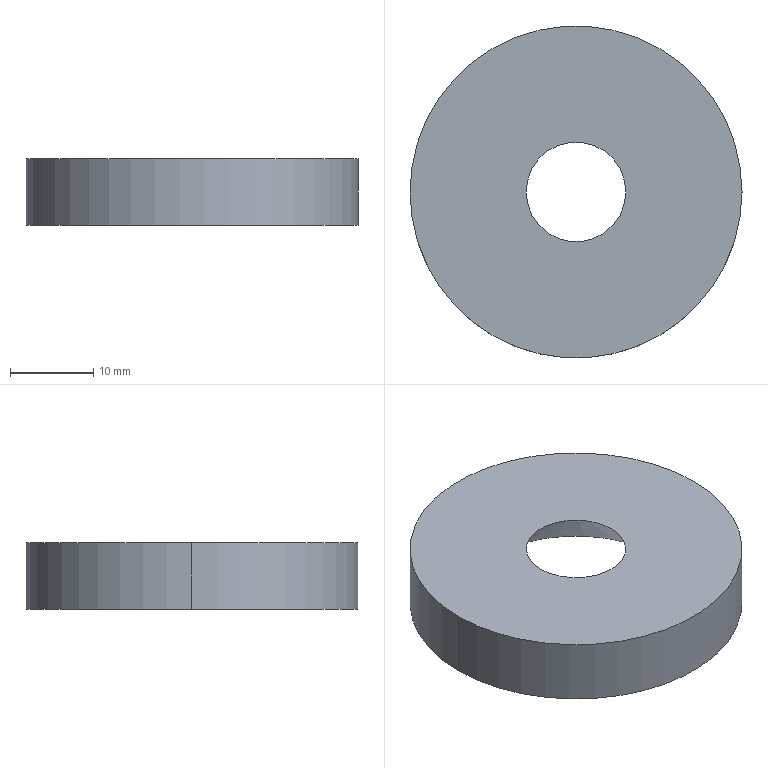Part | STEP file | 1 solid | 6 faces | box 40 x 40 x 8 mm | volume 7406 mm3 | cone 2 | plane 2 | cylinder 2 | commonest cylinder face diameters 40 x2
STEP:
#1=CARTESIAN_POINT('',(0.,0.,0.));
#2=DIRECTION('',(0.,0.,1.));
#3=DIRECTION('',(1.,0.,0.));
#4=AXIS2_PLACEMENT_3D('',#1,#2,#3);
#5=CARTESIAN_POINT('',(-14.,0.,0.));
#6=VERTEX_POINT('',#5);
#7=CARTESIAN_POINT('',(14.,0.,0.));
#8=VERTEX_POINT('',#7);
#9=CARTESIAN_POINT('',(0.,0.,0.));
#10=DIRECTION('',(0.,0.,1.));
#11=DIRECTION('',(1.,0.,0.));
#12=AXIS2_PLACEMENT_3D('',#9,#10,#11);
#13=CIRCLE('',#12,14.);
#14=CARTESIAN_POINT('',(0.,0.,8.));
#15=DIRECTION('',(0.,0.,-1.));
#16=DIRECTION('',(1.,0.,0.));
#17=AXIS2_PLACEMENT_3D('',#14,#15,#16);
#18=CONICAL_SURFACE('',#17,6.,0.7854);
#19=CARTESIAN_POINT('',(6.283,8.));
#20=DIRECTION('',(-1.,0.));
#21=VECTOR('',#20,1.);
#22=LINE('',#19,#21);
#23=(GEOMETRIC_REPRESENTATION_CONTEXT(2)PARAMETRIC_REPRESENTATION_CONTEXT()REPRESENTATION_CONTEXT('',''));
#24=DEFINITIONAL_REPRESENTATION('',(#22),#23);
#25=PCURVE('',#18,#24);
#26=CARTESIAN_POINT('',(0.,0.,0.));
#27=DIRECTION('',(0.,0.,1.));
#28=DIRECTION('',(1.,0.,0.));
#29=AXIS2_PLACEMENT_3D('',#26,#27,#28);
#30=PLANE('',#29);
#31=CARTESIAN_POINT('',(0.,0.));
#32=DIRECTION('',(1.,0.));
#33=AXIS2_PLACEMENT_2D('',#31,#32);
#34=CIRCLE('',#33,14.);
#35=(GEOMETRIC_REPRESENTATION_CONTEXT(2)PARAMETRIC_REPRESENTATION_CONTEXT()REPRESENTATION_CONTEXT('',''));
#36=DEFINITIONAL_REPRESENTATION('',(#34),#35);
#37=PCURVE('',#30,#36);
#38=SURFACE_CURVE('',#13,(#25,#37),.PCURVE_S1.);
#39=EDGE_CURVE('',#6,#8,#38,.T.);
#40=ORIENTED_EDGE('',*,*,#39,.T.);
#41=CARTESIAN_POINT('',(6.,0.,8.));
#42=VERTEX_POINT('',#41);
#43=CARTESIAN_POINT('',(6.,0.,8.));
#44=DIRECTION('',(0.7071,0.,-0.7071));
#45=VECTOR('',#44,1.);
#46=LINE('',#43,#45);
#47=CARTESIAN_POINT('',(0.,0.));
#48=DIRECTION('',(0.,1.));
#49=VECTOR('',#48,1.);
#50=LINE('',#47,#49);
#51=(GEOMETRIC_REPRESENTATION_CONTEXT(2)PARAMETRIC_REPRESENTATION_CONTEXT()REPRESENTATION_CONTEXT('',''));
#52=DEFINITIONAL_REPRESENTATION('',(#50),#51);
#53=PCURVE('',#18,#52);
#54=CARTESIAN_POINT('',(0.,0.,8.));
#55=DIRECTION('',(0.,0.,-1.));
#56=DIRECTION('',(1.,0.,0.));
#57=AXIS2_PLACEMENT_3D('',#54,#55,#56);
#58=CONICAL_SURFACE('',#57,6.,0.7854);
#59=CARTESIAN_POINT('',(6.283,0.));
#60=DIRECTION('',(0.,1.));
#61=VECTOR('',#60,1.);
#62=LINE('',#59,#61);
#63=(GEOMETRIC_REPRESENTATION_CONTEXT(2)PARAMETRIC_REPRESENTATION_CONTEXT()REPRESENTATION_CONTEXT('',''));
#64=DEFINITIONAL_REPRESENTATION('',(#62),#63);
#65=PCURVE('',#58,#64);
#66=SURFACE_CURVE('',#46,(#53,#65),.PCURVE_S1.);
#67=EDGE_CURVE('',#42,#8,#66,.T.);
#68=ORIENTED_EDGE('',*,*,#67,.F.);
#69=CARTESIAN_POINT('',(-6.,0.,8.));
#70=VERTEX_POINT('',#69);
#71=CARTESIAN_POINT('',(0.,0.,8.));
#72=DIRECTION('',(0.,0.,1.));
#73=DIRECTION('',(1.,0.,0.));
#74=AXIS2_PLACEMENT_3D('',#71,#72,#73);
#75=CIRCLE('',#74,6.);
#76=CARTESIAN_POINT('',(6.283,0.));
#77=DIRECTION('',(-1.,0.));
#78=VECTOR('',#77,1.);
#79=LINE('',#76,#78);
#80=(GEOMETRIC_REPRESENTATION_CONTEXT(2)PARAMETRIC_REPRESENTATION_CONTEXT()REPRESENTATION_CONTEXT('',''));
#81=DEFINITIONAL_REPRESENTATION('',(#79),#80);
#82=PCURVE('',#18,#81);
#83=CARTESIAN_POINT('',(0.,0.,8.));
#84=DIRECTION('',(0.,0.,1.));
#85=DIRECTION('',(1.,0.,0.));
#86=AXIS2_PLACEMENT_3D('',#83,#84,#85);
#87=PLANE('',#86);
#88=CARTESIAN_POINT('',(0.,0.));
#89=DIRECTION('',(1.,0.));
#90=AXIS2_PLACEMENT_2D('',#88,#89);
#91=CIRCLE('',#90,6.);
#92=(GEOMETRIC_REPRESENTATION_CONTEXT(2)PARAMETRIC_REPRESENTATION_CONTEXT()REPRESENTATION_CONTEXT('',''));
#93=DEFINITIONAL_REPRESENTATION('',(#91),#92);
#94=PCURVE('',#87,#93);
#95=SURFACE_CURVE('',#75,(#82,#94),.PCURVE_S1.);
#96=EDGE_CURVE('',#70,#42,#95,.T.);
#97=ORIENTED_EDGE('',*,*,#96,.F.);
#98=CARTESIAN_POINT('',(-6.,0.,8.));
#99=DIRECTION('',(-0.7071,0.,-0.7071));
#100=VECTOR('',#99,1.);
#101=LINE('',#98,#100);
#102=CARTESIAN_POINT('',(3.142,0.));
#103=DIRECTION('',(0.,1.));
#104=VECTOR('',#103,1.);
#105=LINE('',#102,#104);
#106=(GEOMETRIC_REPRESENTATION_CONTEXT(2)PARAMETRIC_REPRESENTATION_CONTEXT()REPRESENTATION_CONTEXT('',''));
#107=DEFINITIONAL_REPRESENTATION('',(#105),#106);
#108=PCURVE('',#18,#107);
#109=CARTESIAN_POINT('',(3.142,0.));
#110=DIRECTION('',(0.,1.));
#111=VECTOR('',#110,1.);
#112=LINE('',#109,#111);
#113=(GEOMETRIC_REPRESENTATION_CONTEXT(2)PARAMETRIC_REPRESENTATION_CONTEXT()REPRESENTATION_CONTEXT('',''));
#114=DEFINITIONAL_REPRESENTATION('',(#112),#113);
#115=PCURVE('',#58,#114);
#116=SURFACE_CURVE('',#101,(#108,#115),.PCURVE_S1.);
#117=EDGE_CURVE('',#70,#6,#116,.T.);
#118=ORIENTED_EDGE('',*,*,#117,.T.);
#119=EDGE_LOOP('',(#40,#68,#97,#118));
#120=FACE_BOUND('',#119,.F.);
#121=ADVANCED_FACE('',(#120),#18,.F.);
#122=CARTESIAN_POINT('',(0.,0.,0.));
#123=DIRECTION('',(0.,0.,1.));
#124=DIRECTION('',(1.,0.,0.));
#125=AXIS2_PLACEMENT_3D('',#122,#123,#124);
#126=CIRCLE('',#125,14.);
#127=CARTESIAN_POINT('',(0.,0.));
#128=DIRECTION('',(1.,0.));
#129=AXIS2_PLACEMENT_2D('',#127,#128);
#130=CIRCLE('',#129,14.);
#131=(GEOMETRIC_REPRESENTATION_CONTEXT(2)PARAMETRIC_REPRESENTATION_CONTEXT()REPRESENTATION_CONTEXT('',''));
#132=DEFINITIONAL_REPRESENTATION('',(#130),#131);
#133=PCURVE('',#30,#132);
#134=CARTESIAN_POINT('',(6.283,8.));
#135=DIRECTION('',(-1.,0.));
#136=VECTOR('',#135,1.);
#137=LINE('',#134,#136);
#138=(GEOMETRIC_REPRESENTATION_CONTEXT(2)PARAMETRIC_REPRESENTATION_CONTEXT()REPRESENTATION_CONTEXT('',''));
#139=DEFINITIONAL_REPRESENTATION('',(#137),#138);
#140=PCURVE('',#58,#139);
#141=SURFACE_CURVE('',#126,(#133,#140),.PCURVE_S1.);
#142=EDGE_CURVE('',#8,#6,#141,.T.);
#143=ORIENTED_EDGE('',*,*,#142,.T.);
#144=ORIENTED_EDGE('',*,*,#39,.T.);
#145=EDGE_LOOP('',(#143,#144));
#146=FACE_BOUND('',#145,.T.);
#147=CARTESIAN_POINT('',(-20.,0.,0.));
#148=VERTEX_POINT('',#147);
#149=CARTESIAN_POINT('',(20.,0.,0.));
#150=VERTEX_POINT('',#149);
#151=CARTESIAN_POINT('',(0.,0.,0.));
#152=DIRECTION('',(0.,0.,1.));
#153=DIRECTION('',(1.,0.,0.));
#154=AXIS2_PLACEMENT_3D('',#151,#152,#153);
#155=CIRCLE('',#154,20.);
#156=CARTESIAN_POINT('',(0.,0.));
#157=DIRECTION('',(1.,0.));
#158=AXIS2_PLACEMENT_2D('',#156,#157);
#159=CIRCLE('',#158,20.);
#160=(GEOMETRIC_REPRESENTATION_CONTEXT(2)PARAMETRIC_REPRESENTATION_CONTEXT()REPRESENTATION_CONTEXT('',''));
#161=DEFINITIONAL_REPRESENTATION('',(#159),#160);
#162=PCURVE('',#30,#161);
#163=CARTESIAN_POINT('',(0.,0.,8.));
#164=DIRECTION('',(0.,0.,-1.));
#165=DIRECTION('',(-1.,0.,0.));
#166=AXIS2_PLACEMENT_3D('',#163,#164,#165);
#167=CYLINDRICAL_SURFACE('',#166,20.);
#168=CARTESIAN_POINT('',(9.425,8.));
#169=DIRECTION('',(-1.,0.));
#170=VECTOR('',#169,1.);
#171=LINE('',#168,#170);
#172=(GEOMETRIC_REPRESENTATION_CONTEXT(2)PARAMETRIC_REPRESENTATION_CONTEXT()REPRESENTATION_CONTEXT('',''));
#173=DEFINITIONAL_REPRESENTATION('',(#171),#172);
#174=PCURVE('',#167,#173);
#175=SURFACE_CURVE('',#155,(#162,#174),.PCURVE_S1.);
#176=EDGE_CURVE('',#148,#150,#175,.T.);
#177=ORIENTED_EDGE('',*,*,#176,.F.);
#178=CARTESIAN_POINT('',(0.,0.,0.));
#179=DIRECTION('',(0.,0.,1.));
#180=DIRECTION('',(1.,0.,0.));
#181=AXIS2_PLACEMENT_3D('',#178,#179,#180);
#182=CIRCLE('',#181,20.);
#183=CARTESIAN_POINT('',(0.,0.));
#184=DIRECTION('',(1.,0.));
#185=AXIS2_PLACEMENT_2D('',#183,#184);
#186=CIRCLE('',#185,20.);
#187=(GEOMETRIC_REPRESENTATION_CONTEXT(2)PARAMETRIC_REPRESENTATION_CONTEXT()REPRESENTATION_CONTEXT('',''));
#188=DEFINITIONAL_REPRESENTATION('',(#186),#187);
#189=PCURVE('',#30,#188);
#190=CARTESIAN_POINT('',(0.,0.,8.));
#191=DIRECTION('',(0.,0.,-1.));
#192=DIRECTION('',(-1.,0.,0.));
#193=AXIS2_PLACEMENT_3D('',#190,#191,#192);
#194=CYLINDRICAL_SURFACE('',#193,20.);
#195=CARTESIAN_POINT('',(3.142,8.));
#196=DIRECTION('',(-1.,0.));
#197=VECTOR('',#196,1.);
#198=LINE('',#195,#197);
#199=(GEOMETRIC_REPRESENTATION_CONTEXT(2)PARAMETRIC_REPRESENTATION_CONTEXT()REPRESENTATION_CONTEXT('',''));
#200=DEFINITIONAL_REPRESENTATION('',(#198),#199);
#201=PCURVE('',#194,#200);
#202=SURFACE_CURVE('',#182,(#189,#201),.PCURVE_S1.);
#203=EDGE_CURVE('',#150,#148,#202,.T.);
#204=ORIENTED_EDGE('',*,*,#203,.F.);
#205=EDGE_LOOP('',(#177,#204));
#206=FACE_BOUND('',#205,.T.);
#207=ADVANCED_FACE('',(#146,#206),#30,.F.);
#208=CARTESIAN_POINT('',(0.,0.,8.));
#209=DIRECTION('',(0.,0.,1.));
#210=DIRECTION('',(1.,0.,0.));
#211=AXIS2_PLACEMENT_3D('',#208,#209,#210);
#212=CIRCLE('',#211,6.);
#213=CARTESIAN_POINT('',(0.,0.));
#214=DIRECTION('',(1.,0.));
#215=AXIS2_PLACEMENT_2D('',#213,#214);
#216=CIRCLE('',#215,6.);
#217=(GEOMETRIC_REPRESENTATION_CONTEXT(2)PARAMETRIC_REPRESENTATION_CONTEXT()REPRESENTATION_CONTEXT('',''));
#218=DEFINITIONAL_REPRESENTATION('',(#216),#217);
#219=PCURVE('',#87,#218);
#220=CARTESIAN_POINT('',(6.283,0.));
#221=DIRECTION('',(-1.,0.));
#222=VECTOR('',#221,1.);
#223=LINE('',#220,#222);
#224=(GEOMETRIC_REPRESENTATION_CONTEXT(2)PARAMETRIC_REPRESENTATION_CONTEXT()REPRESENTATION_CONTEXT('',''));
#225=DEFINITIONAL_REPRESENTATION('',(#223),#224);
#226=PCURVE('',#58,#225);
#227=SURFACE_CURVE('',#212,(#219,#226),.PCURVE_S1.);
#228=EDGE_CURVE('',#42,#70,#227,.T.);
#229=ORIENTED_EDGE('',*,*,#228,.F.);
#230=ORIENTED_EDGE('',*,*,#96,.F.);
#231=EDGE_LOOP('',(#229,#230));
#232=FACE_BOUND('',#231,.T.);
#233=CARTESIAN_POINT('',(-20.,0.,8.));
#234=VERTEX_POINT('',#233);
#235=CARTESIAN_POINT('',(20.,0.,8.));
#236=VERTEX_POINT('',#235);
#237=CARTESIAN_POINT('',(0.,0.,8.));
#238=DIRECTION('',(0.,0.,1.));
#239=DIRECTION('',(1.,0.,0.));
#240=AXIS2_PLACEMENT_3D('',#237,#238,#239);
#241=CIRCLE('',#240,20.);
#242=CARTESIAN_POINT('',(0.,0.));
#243=DIRECTION('',(1.,0.));
#244=AXIS2_PLACEMENT_2D('',#242,#243);
#245=CIRCLE('',#244,20.);
#246=(GEOMETRIC_REPRESENTATION_CONTEXT(2)PARAMETRIC_REPRESENTATION_CONTEXT()REPRESENTATION_CONTEXT('',''));
#247=DEFINITIONAL_REPRESENTATION('',(#245),#246);
#248=PCURVE('',#87,#247);
#249=CARTESIAN_POINT('',(9.425,0.));
#250=DIRECTION('',(-1.,0.));
#251=VECTOR('',#250,1.);
#252=LINE('',#249,#251);
#253=(GEOMETRIC_REPRESENTATION_CONTEXT(2)PARAMETRIC_REPRESENTATION_CONTEXT()REPRESENTATION_CONTEXT('',''));
#254=DEFINITIONAL_REPRESENTATION('',(#252),#253);
#255=PCURVE('',#167,#254);
#256=SURFACE_CURVE('',#241,(#248,#255),.PCURVE_S1.);
#257=EDGE_CURVE('',#234,#236,#256,.T.);
#258=ORIENTED_EDGE('',*,*,#257,.T.);
#259=CARTESIAN_POINT('',(0.,0.,8.));
#260=DIRECTION('',(0.,0.,1.));
#261=DIRECTION('',(1.,0.,0.));
#262=AXIS2_PLACEMENT_3D('',#259,#260,#261);
#263=CIRCLE('',#262,20.);
#264=CARTESIAN_POINT('',(0.,0.));
#265=DIRECTION('',(1.,0.));
#266=AXIS2_PLACEMENT_2D('',#264,#265);
#267=CIRCLE('',#266,20.);
#268=(GEOMETRIC_REPRESENTATION_CONTEXT(2)PARAMETRIC_REPRESENTATION_CONTEXT()REPRESENTATION_CONTEXT('',''));
#269=DEFINITIONAL_REPRESENTATION('',(#267),#268);
#270=PCURVE('',#87,#269);
#271=CARTESIAN_POINT('',(3.142,0.));
#272=DIRECTION('',(-1.,0.));
#273=VECTOR('',#272,1.);
#274=LINE('',#271,#273);
#275=(GEOMETRIC_REPRESENTATION_CONTEXT(2)PARAMETRIC_REPRESENTATION_CONTEXT()REPRESENTATION_CONTEXT('',''));
#276=DEFINITIONAL_REPRESENTATION('',(#274),#275);
#277=PCURVE('',#194,#276);
#278=SURFACE_CURVE('',#263,(#270,#277),.PCURVE_S1.);
#279=EDGE_CURVE('',#236,#234,#278,.T.);
#280=ORIENTED_EDGE('',*,*,#279,.T.);
#281=EDGE_LOOP('',(#258,#280));
#282=FACE_BOUND('',#281,.T.);
#283=ADVANCED_FACE('',(#232,#282),#87,.T.);
#284=CARTESIAN_POINT('',(20.,0.,8.));
#285=DIRECTION('',(0.,0.,-1.));
#286=VECTOR('',#285,1.);
#287=LINE('',#284,#286);
#288=CARTESIAN_POINT('',(3.142,0.));
#289=DIRECTION('',(0.,1.));
#290=VECTOR('',#289,1.);
#291=LINE('',#288,#290);
#292=(GEOMETRIC_REPRESENTATION_CONTEXT(2)PARAMETRIC_REPRESENTATION_CONTEXT()REPRESENTATION_CONTEXT('',''));
#293=DEFINITIONAL_REPRESENTATION('',(#291),#292);
#294=PCURVE('',#167,#293);
#295=CARTESIAN_POINT('',(3.142,0.));
#296=DIRECTION('',(0.,1.));
#297=VECTOR('',#296,1.);
#298=LINE('',#295,#297);
#299=(GEOMETRIC_REPRESENTATION_CONTEXT(2)PARAMETRIC_REPRESENTATION_CONTEXT()REPRESENTATION_CONTEXT('',''));
#300=DEFINITIONAL_REPRESENTATION('',(#298),#299);
#301=PCURVE('',#194,#300);
#302=SURFACE_CURVE('',#287,(#294,#301),.PCURVE_S1.);
#303=EDGE_CURVE('',#236,#150,#302,.T.);
#304=ORIENTED_EDGE('',*,*,#303,.F.);
#305=ORIENTED_EDGE('',*,*,#257,.F.);
#306=CARTESIAN_POINT('',(-20.,0.,8.));
#307=DIRECTION('',(0.,0.,-1.));
#308=VECTOR('',#307,1.);
#309=LINE('',#306,#308);
#310=CARTESIAN_POINT('',(6.283,0.));
#311=DIRECTION('',(0.,1.));
#312=VECTOR('',#311,1.);
#313=LINE('',#310,#312);
#314=(GEOMETRIC_REPRESENTATION_CONTEXT(2)PARAMETRIC_REPRESENTATION_CONTEXT()REPRESENTATION_CONTEXT('',''));
#315=DEFINITIONAL_REPRESENTATION('',(#313),#314);
#316=PCURVE('',#167,#315);
#317=CARTESIAN_POINT('',(0.,0.));
#318=DIRECTION('',(0.,1.));
#319=VECTOR('',#318,1.);
#320=LINE('',#317,#319);
#321=(GEOMETRIC_REPRESENTATION_CONTEXT(2)PARAMETRIC_REPRESENTATION_CONTEXT()REPRESENTATION_CONTEXT('',''));
#322=DEFINITIONAL_REPRESENTATION('',(#320),#321);
#323=PCURVE('',#194,#322);
#324=SURFACE_CURVE('',#309,(#316,#323),.PCURVE_S1.);
#325=EDGE_CURVE('',#234,#148,#324,.T.);
#326=ORIENTED_EDGE('',*,*,#325,.T.);
#327=ORIENTED_EDGE('',*,*,#176,.T.);
#328=EDGE_LOOP('',(#304,#305,#326,#327));
#329=FACE_BOUND('',#328,.T.);
#330=ADVANCED_FACE('',(#329),#167,.T.);
#331=ORIENTED_EDGE('',*,*,#279,.F.);
#332=ORIENTED_EDGE('',*,*,#303,.T.);
#333=ORIENTED_EDGE('',*,*,#203,.T.);
#334=ORIENTED_EDGE('',*,*,#325,.F.);
#335=EDGE_LOOP('',(#331,#332,#333,#334));
#336=FACE_BOUND('',#335,.T.);
#337=ADVANCED_FACE('',(#336),#194,.T.);
#338=ORIENTED_EDGE('',*,*,#67,.T.);
#339=ORIENTED_EDGE('',*,*,#142,.T.);
#340=ORIENTED_EDGE('',*,*,#117,.F.);
#341=ORIENTED_EDGE('',*,*,#228,.F.);
#342=EDGE_LOOP('',(#338,#339,#340,#341));
#343=FACE_BOUND('',#342,.F.);
#344=ADVANCED_FACE('',(#343),#58,.F.);
#345=CLOSED_SHELL('',(#121,#207,#283,#330,#337,#344));
#346=MANIFOLD_SOLID_BREP('',#345);
#347=(LENGTH_UNIT()NAMED_UNIT(*)SI_UNIT(.MILLI.,.METRE.));
#348=UNCERTAINTY_MEASURE_WITH_UNIT(LENGTH_MEASURE(0.0000001),#347,'','');
#349=(NAMED_UNIT(*)PLANE_ANGLE_UNIT()SI_UNIT($,.RADIAN.));
#350=(NAMED_UNIT(*)SI_UNIT($,.STERADIAN.)SOLID_ANGLE_UNIT());
#351=(GEOMETRIC_REPRESENTATION_CONTEXT(3)GLOBAL_UNCERTAINTY_ASSIGNED_CONTEXT((#348))GLOBAL_UNIT_ASSIGNED_CONTEXT((#347,#349,#350))REPRESENTATION_CONTEXT('',''));
#352=ADVANCED_BREP_SHAPE_REPRESENTATION('',(#4,#346),#351);